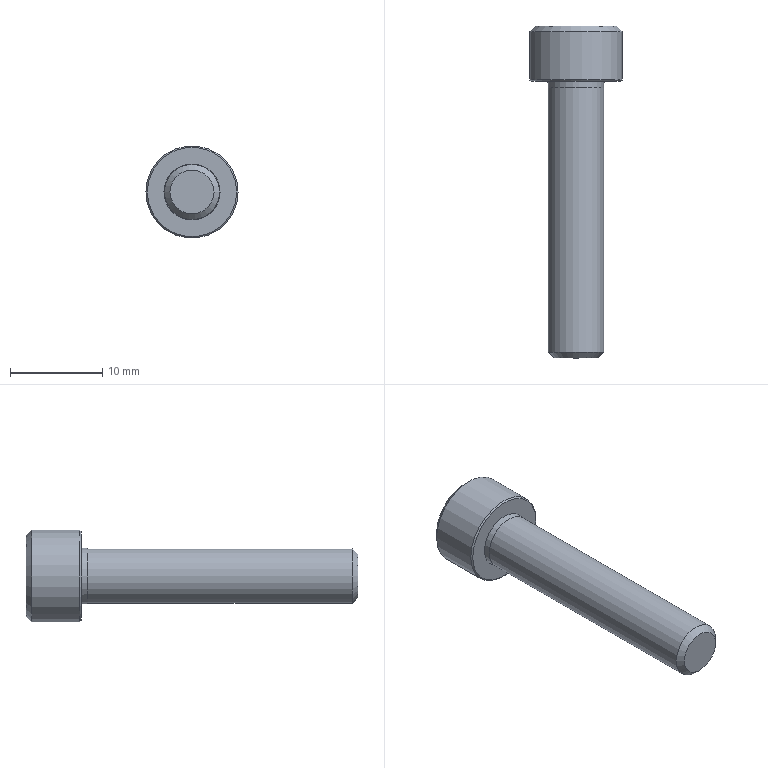Part | STEP file | DIN-912 - M6x30(F) | 1 solid | 28 faces | box 10 x 36 x 10 mm | volume 1236 mm3 | plane 15 | cone 11 | cylinder 2 | commonest cylinder face diameters 6 x1 10 x1